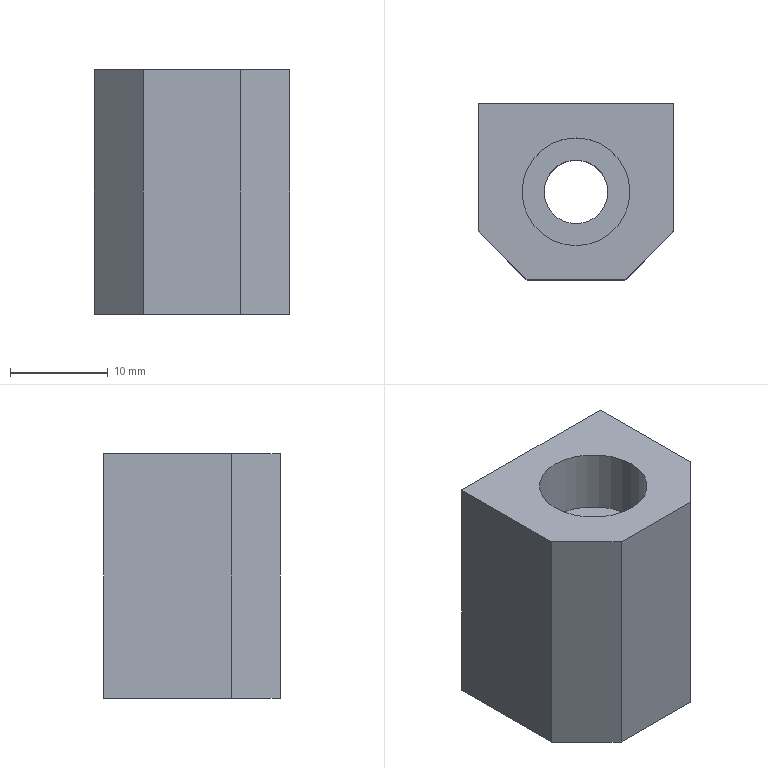Part | STEP file | P011002S004-007 | 1 solid | 11 faces | box 20 x 18 x 25 mm | volume 7143 mm3 | plane 9 | cylinder 2 | commonest cylinder face diameters 6.5 x1 11 x1
STEP:
#1=CARTESIAN_POINT('',(0.,0.,0.));
#2=DIRECTION('',(0.,0.,1.));
#3=DIRECTION('',(1.,0.,0.));
#4=AXIS2_PLACEMENT_3D('',#1,#2,#3);
#5=CARTESIAN_POINT('',(5.,-287.,-23.));
#6=VERTEX_POINT('',#5);
#7=CARTESIAN_POINT('',(-5.,-287.,-23.));
#8=VERTEX_POINT('',#7);
#9=CARTESIAN_POINT('',(-5.,-287.,-23.));
#10=DIRECTION('',(-1.,0.,0.));
#11=VECTOR('',#10,1.);
#12=LINE('',#9,#11);
#13=CARTESIAN_POINT('',(-5.,-274.,-23.));
#14=DIRECTION('',(0.,0.,-1.));
#15=DIRECTION('',(0.,1.,0.));
#16=AXIS2_PLACEMENT_3D('',#13,#14,#15);
#17=PLANE('',#16);
#18=CARTESIAN_POINT('',(-13.,0.));
#19=DIRECTION('',(0.,-1.));
#20=VECTOR('',#19,1.);
#21=LINE('',#18,#20);
#22=(GEOMETRIC_REPRESENTATION_CONTEXT(2)PARAMETRIC_REPRESENTATION_CONTEXT()REPRESENTATION_CONTEXT('',''));
#23=DEFINITIONAL_REPRESENTATION('',(#21),#22);
#24=PCURVE('',#17,#23);
#25=CARTESIAN_POINT('',(-5.,-287.,-23.));
#26=DIRECTION('',(0.,-1.,0.));
#27=DIRECTION('',(0.,0.,-1.));
#28=AXIS2_PLACEMENT_3D('',#25,#26,#27);
#29=PLANE('',#28);
#30=CARTESIAN_POINT('',(0.,0.));
#31=DIRECTION('',(0.,-1.));
#32=VECTOR('',#31,1.);
#33=LINE('',#30,#32);
#34=(GEOMETRIC_REPRESENTATION_CONTEXT(2)PARAMETRIC_REPRESENTATION_CONTEXT()REPRESENTATION_CONTEXT('',''));
#35=DEFINITIONAL_REPRESENTATION('',(#33),#34);
#36=PCURVE('',#29,#35);
#37=SURFACE_CURVE('',#12,(#24,#36),.PCURVE_S1.);
#38=EDGE_CURVE('',#6,#8,#37,.T.);
#39=ORIENTED_EDGE('',*,*,#38,.T.);
#40=CARTESIAN_POINT('',(-10.,-282.,-23.));
#41=VERTEX_POINT('',#40);
#42=CARTESIAN_POINT('',(-11.5,-280.5,-23.));
#43=DIRECTION('',(0.7071,-0.7071,0.));
#44=VECTOR('',#43,1.);
#45=LINE('',#42,#44);
#46=CARTESIAN_POINT('',(-6.5,-6.5));
#47=DIRECTION('',(-0.7071,0.7071));
#48=VECTOR('',#47,1.);
#49=LINE('',#46,#48);
#50=(GEOMETRIC_REPRESENTATION_CONTEXT(2)PARAMETRIC_REPRESENTATION_CONTEXT()REPRESENTATION_CONTEXT('',''));
#51=DEFINITIONAL_REPRESENTATION('',(#49),#50);
#52=PCURVE('',#17,#51);
#53=CARTESIAN_POINT('',(-5.,-287.,-23.));
#54=DIRECTION('',(0.7071,0.7071,0.));
#55=DIRECTION('',(0.7071,-0.7071,0.));
#56=AXIS2_PLACEMENT_3D('',#53,#54,#55);
#57=PLANE('',#56);
#58=CARTESIAN_POINT('',(-9.192,0.));
#59=DIRECTION('',(1.,0.));
#60=VECTOR('',#59,1.);
#61=LINE('',#58,#60);
#62=(GEOMETRIC_REPRESENTATION_CONTEXT(2)PARAMETRIC_REPRESENTATION_CONTEXT()REPRESENTATION_CONTEXT('',''));
#63=DEFINITIONAL_REPRESENTATION('',(#61),#62);
#64=PCURVE('',#57,#63);
#65=SURFACE_CURVE('',#45,(#52,#64),.PCURVE_S1.);
#66=EDGE_CURVE('',#41,#8,#65,.T.);
#67=ORIENTED_EDGE('',*,*,#66,.F.);
#68=CARTESIAN_POINT('',(-10.,-269.,-23.));
#69=VERTEX_POINT('',#68);
#70=CARTESIAN_POINT('',(-10.,-274.,-23.));
#71=DIRECTION('',(0.,1.,0.));
#72=VECTOR('',#71,1.);
#73=LINE('',#70,#72);
#74=CARTESIAN_POINT('',(0.,-5.));
#75=DIRECTION('',(1.,0.));
#76=VECTOR('',#75,1.);
#77=LINE('',#74,#76);
#78=(GEOMETRIC_REPRESENTATION_CONTEXT(2)PARAMETRIC_REPRESENTATION_CONTEXT()REPRESENTATION_CONTEXT('',''));
#79=DEFINITIONAL_REPRESENTATION('',(#77),#78);
#80=PCURVE('',#17,#79);
#81=CARTESIAN_POINT('',(-10.,-274.,-23.));
#82=DIRECTION('',(-1.,0.,0.));
#83=DIRECTION('',(0.,0.,1.));
#84=AXIS2_PLACEMENT_3D('',#81,#82,#83);
#85=PLANE('',#84);
#86=CARTESIAN_POINT('',(0.,0.));
#87=DIRECTION('',(0.,1.));
#88=VECTOR('',#87,1.);
#89=LINE('',#86,#88);
#90=(GEOMETRIC_REPRESENTATION_CONTEXT(2)PARAMETRIC_REPRESENTATION_CONTEXT()REPRESENTATION_CONTEXT('',''));
#91=DEFINITIONAL_REPRESENTATION('',(#89),#90);
#92=PCURVE('',#85,#91);
#93=SURFACE_CURVE('',#73,(#80,#92),.PCURVE_S1.);
#94=EDGE_CURVE('',#41,#69,#93,.T.);
#95=ORIENTED_EDGE('',*,*,#94,.T.);
#96=CARTESIAN_POINT('',(10.,-269.,-23.));
#97=VERTEX_POINT('',#96);
#98=CARTESIAN_POINT('',(-5.,-269.,-23.));
#99=DIRECTION('',(1.,0.,0.));
#100=VECTOR('',#99,1.);
#101=LINE('',#98,#100);
#102=CARTESIAN_POINT('',(5.,0.));
#103=DIRECTION('',(0.,1.));
#104=VECTOR('',#103,1.);
#105=LINE('',#102,#104);
#106=(GEOMETRIC_REPRESENTATION_CONTEXT(2)PARAMETRIC_REPRESENTATION_CONTEXT()REPRESENTATION_CONTEXT('',''));
#107=DEFINITIONAL_REPRESENTATION('',(#105),#106);
#108=PCURVE('',#17,#107);
#109=CARTESIAN_POINT('',(-5.,-269.,-23.));
#110=DIRECTION('',(0.,1.,0.));
#111=DIRECTION('',(0.,0.,1.));
#112=AXIS2_PLACEMENT_3D('',#109,#110,#111);
#113=PLANE('',#112);
#114=CARTESIAN_POINT('',(0.,0.));
#115=DIRECTION('',(0.,1.));
#116=VECTOR('',#115,1.);
#117=LINE('',#114,#116);
#118=(GEOMETRIC_REPRESENTATION_CONTEXT(2)PARAMETRIC_REPRESENTATION_CONTEXT()REPRESENTATION_CONTEXT('',''));
#119=DEFINITIONAL_REPRESENTATION('',(#117),#118);
#120=PCURVE('',#113,#119);
#121=SURFACE_CURVE('',#101,(#108,#120),.PCURVE_S1.);
#122=EDGE_CURVE('',#69,#97,#121,.T.);
#123=ORIENTED_EDGE('',*,*,#122,.T.);
#124=CARTESIAN_POINT('',(10.,-282.,-23.));
#125=VERTEX_POINT('',#124);
#126=CARTESIAN_POINT('',(10.,-274.,-23.));
#127=DIRECTION('',(0.,-1.,0.));
#128=VECTOR('',#127,1.);
#129=LINE('',#126,#128);
#130=CARTESIAN_POINT('',(0.,15.));
#131=DIRECTION('',(-1.,0.));
#132=VECTOR('',#131,1.);
#133=LINE('',#130,#132);
#134=(GEOMETRIC_REPRESENTATION_CONTEXT(2)PARAMETRIC_REPRESENTATION_CONTEXT()REPRESENTATION_CONTEXT('',''));
#135=DEFINITIONAL_REPRESENTATION('',(#133),#134);
#136=PCURVE('',#17,#135);
#137=CARTESIAN_POINT('',(10.,-274.,-23.));
#138=DIRECTION('',(1.,0.,0.));
#139=DIRECTION('',(0.,0.,-1.));
#140=AXIS2_PLACEMENT_3D('',#137,#138,#139);
#141=PLANE('',#140);
#142=CARTESIAN_POINT('',(0.,0.));
#143=DIRECTION('',(0.,-1.));
#144=VECTOR('',#143,1.);
#145=LINE('',#142,#144);
#146=(GEOMETRIC_REPRESENTATION_CONTEXT(2)PARAMETRIC_REPRESENTATION_CONTEXT()REPRESENTATION_CONTEXT('',''));
#147=DEFINITIONAL_REPRESENTATION('',(#145),#146);
#148=PCURVE('',#141,#147);
#149=SURFACE_CURVE('',#129,(#136,#148),.PCURVE_S1.);
#150=EDGE_CURVE('',#97,#125,#149,.T.);
#151=ORIENTED_EDGE('',*,*,#150,.T.);
#152=CARTESIAN_POINT('',(6.5,-285.5,-23.));
#153=DIRECTION('',(0.7071,0.7071,0.));
#154=VECTOR('',#153,1.);
#155=LINE('',#152,#154);
#156=CARTESIAN_POINT('',(-11.5,11.5));
#157=DIRECTION('',(0.7071,0.7071));
#158=VECTOR('',#157,1.);
#159=LINE('',#156,#158);
#160=(GEOMETRIC_REPRESENTATION_CONTEXT(2)PARAMETRIC_REPRESENTATION_CONTEXT()REPRESENTATION_CONTEXT('',''));
#161=DEFINITIONAL_REPRESENTATION('',(#159),#160);
#162=PCURVE('',#17,#161);
#163=CARTESIAN_POINT('',(10.,-282.,-23.));
#164=DIRECTION('',(-0.7071,0.7071,0.));
#165=DIRECTION('',(0.7071,0.7071,0.));
#166=AXIS2_PLACEMENT_3D('',#163,#164,#165);
#167=PLANE('',#166);
#168=CARTESIAN_POINT('',(-4.95,0.));
#169=DIRECTION('',(1.,0.));
#170=VECTOR('',#169,1.);
#171=LINE('',#168,#170);
#172=(GEOMETRIC_REPRESENTATION_CONTEXT(2)PARAMETRIC_REPRESENTATION_CONTEXT()REPRESENTATION_CONTEXT('',''));
#173=DEFINITIONAL_REPRESENTATION('',(#171),#172);
#174=PCURVE('',#167,#173);
#175=SURFACE_CURVE('',#155,(#162,#174),.PCURVE_S1.);
#176=EDGE_CURVE('',#6,#125,#175,.T.);
#177=ORIENTED_EDGE('',*,*,#176,.F.);
#178=EDGE_LOOP('',(#39,#67,#95,#123,#151,#177));
#179=FACE_BOUND('',#178,.T.);
#180=CARTESIAN_POINT('',(3.25,-278.,-23.));
#181=VERTEX_POINT('',#180);
#182=CARTESIAN_POINT('',(0.,-278.,-23.));
#183=DIRECTION('',(0.,0.,-1.));
#184=DIRECTION('',(1.,0.,0.));
#185=AXIS2_PLACEMENT_3D('',#182,#183,#184);
#186=CIRCLE('',#185,3.25);
#187=CARTESIAN_POINT('',(-4.,5.));
#188=DIRECTION('',(0.,1.));
#189=AXIS2_PLACEMENT_2D('',#187,#188);
#190=CIRCLE('',#189,3.25);
#191=(GEOMETRIC_REPRESENTATION_CONTEXT(2)PARAMETRIC_REPRESENTATION_CONTEXT()REPRESENTATION_CONTEXT('',''));
#192=DEFINITIONAL_REPRESENTATION('',(#190),#191);
#193=PCURVE('',#17,#192);
#194=CARTESIAN_POINT('',(0.,-278.,19.));
#195=DIRECTION('',(0.,0.,-1.));
#196=DIRECTION('',(1.,0.,0.));
#197=AXIS2_PLACEMENT_3D('',#194,#195,#196);
#198=CYLINDRICAL_SURFACE('',#197,3.25);
#199=CARTESIAN_POINT('',(0.,42.));
#200=DIRECTION('',(1.,0.));
#201=VECTOR('',#200,1.);
#202=LINE('',#199,#201);
#203=(GEOMETRIC_REPRESENTATION_CONTEXT(2)PARAMETRIC_REPRESENTATION_CONTEXT()REPRESENTATION_CONTEXT('',''));
#204=DEFINITIONAL_REPRESENTATION('',(#202),#203);
#205=PCURVE('',#198,#204);
#206=SURFACE_CURVE('',#186,(#193,#205),.PCURVE_S1.);
#207=EDGE_CURVE('',#181,#181,#206,.T.);
#208=ORIENTED_EDGE('',*,*,#207,.F.);
#209=EDGE_LOOP('',(#208));
#210=FACE_BOUND('',#209,.T.);
#211=ADVANCED_FACE('',(#179,#210),#17,.T.);
#212=CARTESIAN_POINT('',(-5.5,-278.,2.));
#213=VERTEX_POINT('',#212);
#214=CARTESIAN_POINT('',(0.,-278.,2.));
#215=DIRECTION('',(0.,0.,-1.));
#216=DIRECTION('',(-1.,0.,0.));
#217=AXIS2_PLACEMENT_3D('',#214,#215,#216);
#218=CIRCLE('',#217,5.5);
#219=CARTESIAN_POINT('',(-5.,-274.,2.));
#220=DIRECTION('',(0.,0.,1.));
#221=DIRECTION('',(0.,-1.,0.));
#222=AXIS2_PLACEMENT_3D('',#219,#220,#221);
#223=PLANE('',#222);
#224=CARTESIAN_POINT('',(4.,-0.5));
#225=CARTESIAN_POINT('',(-5.526,-0.5));
#226=CARTESIAN_POINT('',(-0.7631,7.75));
#227=CARTESIAN_POINT('',(4.,16.));
#228=CARTESIAN_POINT('',(8.763,7.75));
#229=CARTESIAN_POINT('',(13.526,-0.5));
#230=CARTESIAN_POINT('',(4.,-0.5));
#231=(BOUNDED_CURVE()B_SPLINE_CURVE(2,(#224,#225,#226,#227,#228,#229,#230),.UNSPECIFIED.,.T.,.F.)B_SPLINE_CURVE_WITH_KNOTS((1,2,2,2,2,1),(-2.094,0.,2.094,4.189,6.283,8.378),.UNSPECIFIED.)CURVE()GEOMETRIC_REPRESENTATION_ITEM()RATIONAL_B_SPLINE_CURVE((1.,0.5,1.,0.5,1.,0.5,1.))REPRESENTATION_ITEM(''));
#232=(GEOMETRIC_REPRESENTATION_CONTEXT(2)PARAMETRIC_REPRESENTATION_CONTEXT()REPRESENTATION_CONTEXT('',''));
#233=DEFINITIONAL_REPRESENTATION('',(#231),#232);
#234=PCURVE('',#223,#233);
#235=CARTESIAN_POINT('',(0.,-278.,19.));
#236=DIRECTION('',(0.,0.,-1.));
#237=DIRECTION('',(1.,0.,0.));
#238=AXIS2_PLACEMENT_3D('',#235,#236,#237);
#239=CYLINDRICAL_SURFACE('',#238,5.5);
#240=CARTESIAN_POINT('',(3.142,17.));
#241=DIRECTION('',(1.,0.));
#242=VECTOR('',#241,1.);
#243=LINE('',#240,#242);
#244=(GEOMETRIC_REPRESENTATION_CONTEXT(2)PARAMETRIC_REPRESENTATION_CONTEXT()REPRESENTATION_CONTEXT('',''));
#245=DEFINITIONAL_REPRESENTATION('',(#243),#244);
#246=PCURVE('',#239,#245);
#247=SURFACE_CURVE('',#218,(#234,#246),.PCURVE_S1.);
#248=EDGE_CURVE('',#213,#213,#247,.T.);
#249=ORIENTED_EDGE('',*,*,#248,.T.);
#250=EDGE_LOOP('',(#249));
#251=FACE_BOUND('',#250,.T.);
#252=CARTESIAN_POINT('',(10.,-282.,2.));
#253=VERTEX_POINT('',#252);
#254=CARTESIAN_POINT('',(10.,-269.,2.));
#255=VERTEX_POINT('',#254);
#256=CARTESIAN_POINT('',(10.,-274.,2.));
#257=DIRECTION('',(0.,1.,0.));
#258=VECTOR('',#257,1.);
#259=LINE('',#256,#258);
#260=CARTESIAN_POINT('',(0.,15.));
#261=DIRECTION('',(-1.,0.));
#262=VECTOR('',#261,1.);
#263=LINE('',#260,#262);
#264=(GEOMETRIC_REPRESENTATION_CONTEXT(2)PARAMETRIC_REPRESENTATION_CONTEXT()REPRESENTATION_CONTEXT('',''));
#265=DEFINITIONAL_REPRESENTATION('',(#263),#264);
#266=PCURVE('',#223,#265);
#267=CARTESIAN_POINT('',(-25.,0.));
#268=DIRECTION('',(0.,1.));
#269=VECTOR('',#268,1.);
#270=LINE('',#267,#269);
#271=(GEOMETRIC_REPRESENTATION_CONTEXT(2)PARAMETRIC_REPRESENTATION_CONTEXT()REPRESENTATION_CONTEXT('',''));
#272=DEFINITIONAL_REPRESENTATION('',(#270),#271);
#273=PCURVE('',#141,#272);
#274=SURFACE_CURVE('',#259,(#266,#273),.PCURVE_S1.);
#275=EDGE_CURVE('',#253,#255,#274,.T.);
#276=ORIENTED_EDGE('',*,*,#275,.T.);
#277=CARTESIAN_POINT('',(-10.,-269.,2.));
#278=VERTEX_POINT('',#277);
#279=CARTESIAN_POINT('',(-5.,-269.,2.));
#280=DIRECTION('',(-1.,0.,0.));
#281=VECTOR('',#280,1.);
#282=LINE('',#279,#281);
#283=CARTESIAN_POINT('',(-5.,0.));
#284=DIRECTION('',(0.,-1.));
#285=VECTOR('',#284,1.);
#286=LINE('',#283,#285);
#287=(GEOMETRIC_REPRESENTATION_CONTEXT(2)PARAMETRIC_REPRESENTATION_CONTEXT()REPRESENTATION_CONTEXT('',''));
#288=DEFINITIONAL_REPRESENTATION('',(#286),#287);
#289=PCURVE('',#223,#288);
#290=CARTESIAN_POINT('',(25.,0.));
#291=DIRECTION('',(0.,-1.));
#292=VECTOR('',#291,1.);
#293=LINE('',#290,#292);
#294=(GEOMETRIC_REPRESENTATION_CONTEXT(2)PARAMETRIC_REPRESENTATION_CONTEXT()REPRESENTATION_CONTEXT('',''));
#295=DEFINITIONAL_REPRESENTATION('',(#293),#294);
#296=PCURVE('',#113,#295);
#297=SURFACE_CURVE('',#282,(#289,#296),.PCURVE_S1.);
#298=EDGE_CURVE('',#255,#278,#297,.T.);
#299=ORIENTED_EDGE('',*,*,#298,.T.);
#300=CARTESIAN_POINT('',(-10.,-282.,2.));
#301=VERTEX_POINT('',#300);
#302=CARTESIAN_POINT('',(-10.,-274.,2.));
#303=DIRECTION('',(0.,-1.,0.));
#304=VECTOR('',#303,1.);
#305=LINE('',#302,#304);
#306=CARTESIAN_POINT('',(0.,-5.));
#307=DIRECTION('',(1.,0.));
#308=VECTOR('',#307,1.);
#309=LINE('',#306,#308);
#310=(GEOMETRIC_REPRESENTATION_CONTEXT(2)PARAMETRIC_REPRESENTATION_CONTEXT()REPRESENTATION_CONTEXT('',''));
#311=DEFINITIONAL_REPRESENTATION('',(#309),#310);
#312=PCURVE('',#223,#311);
#313=CARTESIAN_POINT('',(25.,0.));
#314=DIRECTION('',(0.,-1.));
#315=VECTOR('',#314,1.);
#316=LINE('',#313,#315);
#317=(GEOMETRIC_REPRESENTATION_CONTEXT(2)PARAMETRIC_REPRESENTATION_CONTEXT()REPRESENTATION_CONTEXT('',''));
#318=DEFINITIONAL_REPRESENTATION('',(#316),#317);
#319=PCURVE('',#85,#318);
#320=SURFACE_CURVE('',#305,(#312,#319),.PCURVE_S1.);
#321=EDGE_CURVE('',#278,#301,#320,.T.);
#322=ORIENTED_EDGE('',*,*,#321,.T.);
#323=CARTESIAN_POINT('',(-5.,-287.,2.));
#324=VERTEX_POINT('',#323);
#325=CARTESIAN_POINT('',(-11.5,-280.5,2.));
#326=DIRECTION('',(-0.7071,0.7071,0.));
#327=VECTOR('',#326,1.);
#328=LINE('',#325,#327);
#329=CARTESIAN_POINT('',(6.5,-6.5));
#330=DIRECTION('',(-0.7071,-0.7071));
#331=VECTOR('',#330,1.);
#332=LINE('',#329,#331);
#333=(GEOMETRIC_REPRESENTATION_CONTEXT(2)PARAMETRIC_REPRESENTATION_CONTEXT()REPRESENTATION_CONTEXT('',''));
#334=DEFINITIONAL_REPRESENTATION('',(#332),#333);
#335=PCURVE('',#223,#334);
#336=CARTESIAN_POINT('',(-9.192,-25.));
#337=DIRECTION('',(-1.,0.));
#338=VECTOR('',#337,1.);
#339=LINE('',#336,#338);
#340=(GEOMETRIC_REPRESENTATION_CONTEXT(2)PARAMETRIC_REPRESENTATION_CONTEXT()REPRESENTATION_CONTEXT('',''));
#341=DEFINITIONAL_REPRESENTATION('',(#339),#340);
#342=PCURVE('',#57,#341);
#343=SURFACE_CURVE('',#328,(#335,#342),.PCURVE_S1.);
#344=EDGE_CURVE('',#324,#301,#343,.T.);
#345=ORIENTED_EDGE('',*,*,#344,.F.);
#346=CARTESIAN_POINT('',(5.,-287.,2.));
#347=VERTEX_POINT('',#346);
#348=CARTESIAN_POINT('',(-5.,-287.,2.));
#349=DIRECTION('',(1.,0.,0.));
#350=VECTOR('',#349,1.);
#351=LINE('',#348,#350);
#352=CARTESIAN_POINT('',(13.,0.));
#353=DIRECTION('',(0.,1.));
#354=VECTOR('',#353,1.);
#355=LINE('',#352,#354);
#356=(GEOMETRIC_REPRESENTATION_CONTEXT(2)PARAMETRIC_REPRESENTATION_CONTEXT()REPRESENTATION_CONTEXT('',''));
#357=DEFINITIONAL_REPRESENTATION('',(#355),#356);
#358=PCURVE('',#223,#357);
#359=CARTESIAN_POINT('',(-25.,0.));
#360=DIRECTION('',(0.,1.));
#361=VECTOR('',#360,1.);
#362=LINE('',#359,#361);
#363=(GEOMETRIC_REPRESENTATION_CONTEXT(2)PARAMETRIC_REPRESENTATION_CONTEXT()REPRESENTATION_CONTEXT('',''));
#364=DEFINITIONAL_REPRESENTATION('',(#362),#363);
#365=PCURVE('',#29,#364);
#366=SURFACE_CURVE('',#351,(#358,#365),.PCURVE_S1.);
#367=EDGE_CURVE('',#324,#347,#366,.T.);
#368=ORIENTED_EDGE('',*,*,#367,.T.);
#369=CARTESIAN_POINT('',(6.5,-285.5,2.));
#370=DIRECTION('',(-0.7071,-0.7071,0.));
#371=VECTOR('',#370,1.);
#372=LINE('',#369,#371);
#373=CARTESIAN_POINT('',(11.5,11.5));
#374=DIRECTION('',(0.7071,-0.7071));
#375=VECTOR('',#374,1.);
#376=LINE('',#373,#375);
#377=(GEOMETRIC_REPRESENTATION_CONTEXT(2)PARAMETRIC_REPRESENTATION_CONTEXT()REPRESENTATION_CONTEXT('',''));
#378=DEFINITIONAL_REPRESENTATION('',(#376),#377);
#379=PCURVE('',#223,#378);
#380=CARTESIAN_POINT('',(-4.95,-25.));
#381=DIRECTION('',(-1.,0.));
#382=VECTOR('',#381,1.);
#383=LINE('',#380,#382);
#384=(GEOMETRIC_REPRESENTATION_CONTEXT(2)PARAMETRIC_REPRESENTATION_CONTEXT()REPRESENTATION_CONTEXT('',''));
#385=DEFINITIONAL_REPRESENTATION('',(#383),#384);
#386=PCURVE('',#167,#385);
#387=SURFACE_CURVE('',#372,(#379,#386),.PCURVE_S1.);
#388=EDGE_CURVE('',#253,#347,#387,.T.);
#389=ORIENTED_EDGE('',*,*,#388,.F.);
#390=EDGE_LOOP('',(#276,#299,#322,#345,#368,#389));
#391=FACE_BOUND('',#390,.T.);
#392=ADVANCED_FACE('',(#251,#391),#223,.T.);
#393=ORIENTED_EDGE('',*,*,#150,.F.);
#394=CARTESIAN_POINT('',(10.,-269.,-23.));
#395=DIRECTION('',(0.,0.,1.));
#396=VECTOR('',#395,1.);
#397=LINE('',#394,#396);
#398=CARTESIAN_POINT('',(0.,5.));
#399=DIRECTION('',(-1.,0.));
#400=VECTOR('',#399,1.);
#401=LINE('',#398,#400);
#402=(GEOMETRIC_REPRESENTATION_CONTEXT(2)PARAMETRIC_REPRESENTATION_CONTEXT()REPRESENTATION_CONTEXT('',''));
#403=DEFINITIONAL_REPRESENTATION('',(#401),#402);
#404=PCURVE('',#141,#403);
#405=CARTESIAN_POINT('',(0.,15.));
#406=DIRECTION('',(1.,0.));
#407=VECTOR('',#406,1.);
#408=LINE('',#405,#407);
#409=(GEOMETRIC_REPRESENTATION_CONTEXT(2)PARAMETRIC_REPRESENTATION_CONTEXT()REPRESENTATION_CONTEXT('',''));
#410=DEFINITIONAL_REPRESENTATION('',(#408),#409);
#411=PCURVE('',#113,#410);
#412=SURFACE_CURVE('',#397,(#404,#411),.PCURVE_S1.);
#413=EDGE_CURVE('',#97,#255,#412,.T.);
#414=ORIENTED_EDGE('',*,*,#413,.T.);
#415=ORIENTED_EDGE('',*,*,#275,.F.);
#416=CARTESIAN_POINT('',(10.,-282.,-23.));
#417=DIRECTION('',(0.,0.,1.));
#418=VECTOR('',#417,1.);
#419=LINE('',#416,#418);
#420=CARTESIAN_POINT('',(0.,-8.));
#421=DIRECTION('',(-1.,0.));
#422=VECTOR('',#421,1.);
#423=LINE('',#420,#422);
#424=(GEOMETRIC_REPRESENTATION_CONTEXT(2)PARAMETRIC_REPRESENTATION_CONTEXT()REPRESENTATION_CONTEXT('',''));
#425=DEFINITIONAL_REPRESENTATION('',(#423),#424);
#426=PCURVE('',#141,#425);
#427=CARTESIAN_POINT('',(0.,0.));
#428=DIRECTION('',(0.,-1.));
#429=VECTOR('',#428,1.);
#430=LINE('',#427,#429);
#431=(GEOMETRIC_REPRESENTATION_CONTEXT(2)PARAMETRIC_REPRESENTATION_CONTEXT()REPRESENTATION_CONTEXT('',''));
#432=DEFINITIONAL_REPRESENTATION('',(#430),#431);
#433=PCURVE('',#167,#432);
#434=SURFACE_CURVE('',#419,(#426,#433),.PCURVE_S1.);
#435=EDGE_CURVE('',#125,#253,#434,.T.);
#436=ORIENTED_EDGE('',*,*,#435,.F.);
#437=EDGE_LOOP('',(#393,#414,#415,#436));
#438=FACE_BOUND('',#437,.T.);
#439=ADVANCED_FACE('',(#438),#141,.T.);
#440=ORIENTED_EDGE('',*,*,#413,.F.);
#441=ORIENTED_EDGE('',*,*,#122,.F.);
#442=CARTESIAN_POINT('',(-10.,-269.,-23.));
#443=DIRECTION('',(0.,0.,1.));
#444=VECTOR('',#443,1.);
#445=LINE('',#442,#444);
#446=CARTESIAN_POINT('',(0.,-5.));
#447=DIRECTION('',(1.,0.));
#448=VECTOR('',#447,1.);
#449=LINE('',#446,#448);
#450=(GEOMETRIC_REPRESENTATION_CONTEXT(2)PARAMETRIC_REPRESENTATION_CONTEXT()REPRESENTATION_CONTEXT('',''));
#451=DEFINITIONAL_REPRESENTATION('',(#449),#450);
#452=PCURVE('',#113,#451);
#453=CARTESIAN_POINT('',(0.,5.));
#454=DIRECTION('',(1.,0.));
#455=VECTOR('',#454,1.);
#456=LINE('',#453,#455);
#457=(GEOMETRIC_REPRESENTATION_CONTEXT(2)PARAMETRIC_REPRESENTATION_CONTEXT()REPRESENTATION_CONTEXT('',''));
#458=DEFINITIONAL_REPRESENTATION('',(#456),#457);
#459=PCURVE('',#85,#458);
#460=SURFACE_CURVE('',#445,(#452,#459),.PCURVE_S1.);
#461=EDGE_CURVE('',#69,#278,#460,.T.);
#462=ORIENTED_EDGE('',*,*,#461,.T.);
#463=ORIENTED_EDGE('',*,*,#298,.F.);
#464=EDGE_LOOP('',(#440,#441,#462,#463));
#465=FACE_BOUND('',#464,.T.);
#466=ADVANCED_FACE('',(#465),#113,.T.);
#467=ORIENTED_EDGE('',*,*,#321,.F.);
#468=ORIENTED_EDGE('',*,*,#461,.F.);
#469=ORIENTED_EDGE('',*,*,#94,.F.);
#470=CARTESIAN_POINT('',(-10.,-282.,-23.));
#471=DIRECTION('',(0.,0.,-1.));
#472=VECTOR('',#471,1.);
#473=LINE('',#470,#472);
#474=CARTESIAN_POINT('',(0.,-8.));
#475=DIRECTION('',(-1.,0.));
#476=VECTOR('',#475,1.);
#477=LINE('',#474,#476);
#478=(GEOMETRIC_REPRESENTATION_CONTEXT(2)PARAMETRIC_REPRESENTATION_CONTEXT()REPRESENTATION_CONTEXT('',''));
#479=DEFINITIONAL_REPRESENTATION('',(#477),#478);
#480=PCURVE('',#85,#479);
#481=CARTESIAN_POINT('',(-7.071,0.));
#482=DIRECTION('',(0.,1.));
#483=VECTOR('',#482,1.);
#484=LINE('',#481,#483);
#485=(GEOMETRIC_REPRESENTATION_CONTEXT(2)PARAMETRIC_REPRESENTATION_CONTEXT()REPRESENTATION_CONTEXT('',''));
#486=DEFINITIONAL_REPRESENTATION('',(#484),#485);
#487=PCURVE('',#57,#486);
#488=SURFACE_CURVE('',#473,(#480,#487),.PCURVE_S1.);
#489=EDGE_CURVE('',#301,#41,#488,.T.);
#490=ORIENTED_EDGE('',*,*,#489,.F.);
#491=EDGE_LOOP('',(#467,#468,#469,#490));
#492=FACE_BOUND('',#491,.T.);
#493=ADVANCED_FACE('',(#492),#85,.T.);
#494=ORIENTED_EDGE('',*,*,#367,.F.);
#495=CARTESIAN_POINT('',(-5.,-287.,-23.));
#496=DIRECTION('',(0.,0.,1.));
#497=VECTOR('',#496,1.);
#498=LINE('',#495,#497);
#499=CARTESIAN_POINT('',(0.,0.));
#500=DIRECTION('',(-1.,0.));
#501=VECTOR('',#500,1.);
#502=LINE('',#499,#501);
#503=(GEOMETRIC_REPRESENTATION_CONTEXT(2)PARAMETRIC_REPRESENTATION_CONTEXT()REPRESENTATION_CONTEXT('',''));
#504=DEFINITIONAL_REPRESENTATION('',(#502),#503);
#505=PCURVE('',#29,#504);
#506=CARTESIAN_POINT('',(0.,0.));
#507=DIRECTION('',(0.,-1.));
#508=VECTOR('',#507,1.);
#509=LINE('',#506,#508);
#510=(GEOMETRIC_REPRESENTATION_CONTEXT(2)PARAMETRIC_REPRESENTATION_CONTEXT()REPRESENTATION_CONTEXT('',''));
#511=DEFINITIONAL_REPRESENTATION('',(#509),#510);
#512=PCURVE('',#57,#511);
#513=SURFACE_CURVE('',#498,(#505,#512),.PCURVE_S1.);
#514=EDGE_CURVE('',#8,#324,#513,.T.);
#515=ORIENTED_EDGE('',*,*,#514,.F.);
#516=ORIENTED_EDGE('',*,*,#38,.F.);
#517=CARTESIAN_POINT('',(5.,-287.,-23.));
#518=DIRECTION('',(0.,0.,-1.));
#519=VECTOR('',#518,1.);
#520=LINE('',#517,#519);
#521=CARTESIAN_POINT('',(0.,10.));
#522=DIRECTION('',(1.,0.));
#523=VECTOR('',#522,1.);
#524=LINE('',#521,#523);
#525=(GEOMETRIC_REPRESENTATION_CONTEXT(2)PARAMETRIC_REPRESENTATION_CONTEXT()REPRESENTATION_CONTEXT('',''));
#526=DEFINITIONAL_REPRESENTATION('',(#524),#525);
#527=PCURVE('',#29,#526);
#528=CARTESIAN_POINT('',(-7.071,0.));
#529=DIRECTION('',(0.,1.));
#530=VECTOR('',#529,1.);
#531=LINE('',#528,#530);
#532=(GEOMETRIC_REPRESENTATION_CONTEXT(2)PARAMETRIC_REPRESENTATION_CONTEXT()REPRESENTATION_CONTEXT('',''));
#533=DEFINITIONAL_REPRESENTATION('',(#531),#532);
#534=PCURVE('',#167,#533);
#535=SURFACE_CURVE('',#520,(#527,#534),.PCURVE_S1.);
#536=EDGE_CURVE('',#347,#6,#535,.T.);
#537=ORIENTED_EDGE('',*,*,#536,.F.);
#538=EDGE_LOOP('',(#494,#515,#516,#537));
#539=FACE_BOUND('',#538,.T.);
#540=ADVANCED_FACE('',(#539),#29,.T.);
#541=ORIENTED_EDGE('',*,*,#176,.T.);
#542=ORIENTED_EDGE('',*,*,#435,.T.);
#543=ORIENTED_EDGE('',*,*,#388,.T.);
#544=ORIENTED_EDGE('',*,*,#536,.T.);
#545=EDGE_LOOP('',(#541,#542,#543,#544));
#546=FACE_BOUND('',#545,.T.);
#547=ADVANCED_FACE('',(#546),#167,.F.);
#548=ORIENTED_EDGE('',*,*,#66,.T.);
#549=ORIENTED_EDGE('',*,*,#514,.T.);
#550=ORIENTED_EDGE('',*,*,#344,.T.);
#551=ORIENTED_EDGE('',*,*,#489,.T.);
#552=EDGE_LOOP('',(#548,#549,#550,#551));
#553=FACE_BOUND('',#552,.T.);
#554=ADVANCED_FACE('',(#553),#57,.F.);
#555=ORIENTED_EDGE('',*,*,#207,.F.);
#556=CARTESIAN_POINT('',(3.25,-278.,-4.5));
#557=VERTEX_POINT('',#556);
#558=CARTESIAN_POINT('',(3.25,-278.,-4.5));
#559=CARTESIAN_POINT('',(3.25,-278.,-23.));
#560=B_SPLINE_CURVE_WITH_KNOTS('',1,(#558,#559),.UNSPECIFIED.,.F.,.F.,(2,2),(23.5,42.),.PIECEWISE_BEZIER_KNOTS.);
#561=CARTESIAN_POINT('',(0.,0.));
#562=DIRECTION('',(0.,1.));
#563=VECTOR('',#562,1.);
#564=LINE('',#561,#563);
#565=(GEOMETRIC_REPRESENTATION_CONTEXT(2)PARAMETRIC_REPRESENTATION_CONTEXT()REPRESENTATION_CONTEXT('',''));
#566=DEFINITIONAL_REPRESENTATION('',(#564),#565);
#567=PCURVE('',#198,#566);
#568=CARTESIAN_POINT('',(6.283,0.));
#569=DIRECTION('',(0.,1.));
#570=VECTOR('',#569,1.);
#571=LINE('',#568,#570);
#572=(GEOMETRIC_REPRESENTATION_CONTEXT(2)PARAMETRIC_REPRESENTATION_CONTEXT()REPRESENTATION_CONTEXT('',''));
#573=DEFINITIONAL_REPRESENTATION('',(#571),#572);
#574=PCURVE('',#198,#573);
#575=SEAM_CURVE('',#560,(#567,#574),.PCURVE_S1.);
#576=EDGE_CURVE('',#557,#181,#575,.T.);
#577=ORIENTED_EDGE('',*,*,#576,.F.);
#578=CARTESIAN_POINT('',(-3.25,-278.,-4.5));
#579=VERTEX_POINT('',#578);
#580=CARTESIAN_POINT('',(0.,-278.,-4.5));
#581=DIRECTION('',(0.,0.,-1.));
#582=DIRECTION('',(-1.,0.,0.));
#583=AXIS2_PLACEMENT_3D('',#580,#581,#582);
#584=CIRCLE('',#583,3.25);
#585=CARTESIAN_POINT('',(-3.142,23.5));
#586=DIRECTION('',(1.,0.));
#587=VECTOR('',#586,1.);
#588=LINE('',#585,#587);
#589=(GEOMETRIC_REPRESENTATION_CONTEXT(2)PARAMETRIC_REPRESENTATION_CONTEXT()REPRESENTATION_CONTEXT('',''));
#590=DEFINITIONAL_REPRESENTATION('',(#588),#589);
#591=PCURVE('',#198,#590);
#592=CARTESIAN_POINT('',(0.,-278.,-4.5));
#593=DIRECTION('',(0.,0.,1.));
#594=DIRECTION('',(-1.,0.,0.));
#595=AXIS2_PLACEMENT_3D('',#592,#593,#594);
#596=PLANE('',#595);
#597=CARTESIAN_POINT('',(3.25,0.));
#598=CARTESIAN_POINT('',(3.25,-5.629));
#599=CARTESIAN_POINT('',(-1.625,-2.815));
#600=CARTESIAN_POINT('',(-6.5,0.));
#601=CARTESIAN_POINT('',(-1.625,2.815));
#602=CARTESIAN_POINT('',(3.25,5.629));
#603=CARTESIAN_POINT('',(3.25,0.));
#604=(BOUNDED_CURVE()B_SPLINE_CURVE(2,(#597,#598,#599,#600,#601,#602,#603),.UNSPECIFIED.,.T.,.F.)B_SPLINE_CURVE_WITH_KNOTS((1,2,2,2,2,1),(-2.094,0.,2.094,4.189,6.283,8.378),.UNSPECIFIED.)CURVE()GEOMETRIC_REPRESENTATION_ITEM()RATIONAL_B_SPLINE_CURVE((1.,0.5,1.,0.5,1.,0.5,1.))REPRESENTATION_ITEM(''));
#605=(GEOMETRIC_REPRESENTATION_CONTEXT(2)PARAMETRIC_REPRESENTATION_CONTEXT()REPRESENTATION_CONTEXT('',''));
#606=DEFINITIONAL_REPRESENTATION('',(#604),#605);
#607=PCURVE('',#596,#606);
#608=SURFACE_CURVE('',#584,(#591,#607),.PCURVE_S1.);
#609=EDGE_CURVE('',#557,#579,#608,.T.);
#610=ORIENTED_EDGE('',*,*,#609,.T.);
#611=CARTESIAN_POINT('',(0.,-278.,-4.5));
#612=DIRECTION('',(0.,0.,-1.));
#613=DIRECTION('',(-1.,0.,0.));
#614=AXIS2_PLACEMENT_3D('',#611,#612,#613);
#615=CIRCLE('',#614,3.25);
#616=CARTESIAN_POINT('',(3.142,23.5));
#617=DIRECTION('',(1.,0.));
#618=VECTOR('',#617,1.);
#619=LINE('',#616,#618);
#620=(GEOMETRIC_REPRESENTATION_CONTEXT(2)PARAMETRIC_REPRESENTATION_CONTEXT()REPRESENTATION_CONTEXT('',''));
#621=DEFINITIONAL_REPRESENTATION('',(#619),#620);
#622=PCURVE('',#198,#621);
#623=CARTESIAN_POINT('',(3.25,0.));
#624=CARTESIAN_POINT('',(3.25,-5.629));
#625=CARTESIAN_POINT('',(-1.625,-2.815));
#626=CARTESIAN_POINT('',(-6.5,0.));
#627=CARTESIAN_POINT('',(-1.625,2.815));
#628=CARTESIAN_POINT('',(3.25,5.629));
#629=CARTESIAN_POINT('',(3.25,0.));
#630=(BOUNDED_CURVE()B_SPLINE_CURVE(2,(#623,#624,#625,#626,#627,#628,#629),.UNSPECIFIED.,.T.,.F.)B_SPLINE_CURVE_WITH_KNOTS((1,2,2,2,2,1),(-2.094,0.,2.094,4.189,6.283,8.378),.UNSPECIFIED.)CURVE()GEOMETRIC_REPRESENTATION_ITEM()RATIONAL_B_SPLINE_CURVE((1.,0.5,1.,0.5,1.,0.5,1.))REPRESENTATION_ITEM(''));
#631=(GEOMETRIC_REPRESENTATION_CONTEXT(2)PARAMETRIC_REPRESENTATION_CONTEXT()REPRESENTATION_CONTEXT('',''));
#632=DEFINITIONAL_REPRESENTATION('',(#630),#631);
#633=PCURVE('',#596,#632);
#634=SURFACE_CURVE('',#615,(#622,#633),.PCURVE_S1.);
#635=EDGE_CURVE('',#579,#557,#634,.T.);
#636=ORIENTED_EDGE('',*,*,#635,.T.);
#637=ORIENTED_EDGE('',*,*,#576,.T.);
#638=EDGE_LOOP('',(#555,#577,#610,#636,#637));
#639=FACE_BOUND('',#638,.F.);
#640=ADVANCED_FACE('',(#639),#198,.F.);
#641=CARTESIAN_POINT('',(-5.5,-278.,-4.5));
#642=VERTEX_POINT('',#641);
#643=CARTESIAN_POINT('',(0.,-278.,-4.5));
#644=DIRECTION('',(0.,0.,-1.));
#645=DIRECTION('',(-1.,0.,0.));
#646=AXIS2_PLACEMENT_3D('',#643,#644,#645);
#647=CIRCLE('',#646,5.5);
#648=CARTESIAN_POINT('',(5.5,0.));
#649=CARTESIAN_POINT('',(5.5,-9.526));
#650=CARTESIAN_POINT('',(-2.75,-4.763));
#651=CARTESIAN_POINT('',(-11.,0.));
#652=CARTESIAN_POINT('',(-2.75,4.763));
#653=CARTESIAN_POINT('',(5.5,9.526));
#654=CARTESIAN_POINT('',(5.5,0.));
#655=(BOUNDED_CURVE()B_SPLINE_CURVE(2,(#648,#649,#650,#651,#652,#653,#654),.UNSPECIFIED.,.T.,.F.)B_SPLINE_CURVE_WITH_KNOTS((1,2,2,2,2,1),(-2.094,0.,2.094,4.189,6.283,8.378),.UNSPECIFIED.)CURVE()GEOMETRIC_REPRESENTATION_ITEM()RATIONAL_B_SPLINE_CURVE((1.,0.5,1.,0.5,1.,0.5,1.))REPRESENTATION_ITEM(''));
#656=(GEOMETRIC_REPRESENTATION_CONTEXT(2)PARAMETRIC_REPRESENTATION_CONTEXT()REPRESENTATION_CONTEXT('',''));
#657=DEFINITIONAL_REPRESENTATION('',(#655),#656);
#658=PCURVE('',#596,#657);
#659=CARTESIAN_POINT('',(3.142,23.5));
#660=DIRECTION('',(1.,0.));
#661=VECTOR('',#660,1.);
#662=LINE('',#659,#661);
#663=(GEOMETRIC_REPRESENTATION_CONTEXT(2)PARAMETRIC_REPRESENTATION_CONTEXT()REPRESENTATION_CONTEXT('',''));
#664=DEFINITIONAL_REPRESENTATION('',(#662),#663);
#665=PCURVE('',#239,#664);
#666=SURFACE_CURVE('',#647,(#658,#665),.PCURVE_S1.);
#667=EDGE_CURVE('',#642,#642,#666,.T.);
#668=ORIENTED_EDGE('',*,*,#667,.F.);
#669=EDGE_LOOP('',(#668));
#670=FACE_BOUND('',#669,.T.);
#671=ORIENTED_EDGE('',*,*,#635,.T.);
#672=ORIENTED_EDGE('',*,*,#609,.T.);
#673=EDGE_LOOP('',(#671,#672));
#674=FACE_BOUND('',#673,.T.);
#675=ADVANCED_FACE('',(#670,#674),#596,.T.);
#676=ORIENTED_EDGE('',*,*,#667,.F.);
#677=CARTESIAN_POINT('',(-5.5,-278.,2.));
#678=CARTESIAN_POINT('',(-5.5,-278.,-4.5));
#679=B_SPLINE_CURVE_WITH_KNOTS('',1,(#677,#678),.UNSPECIFIED.,.F.,.F.,(2,2),(17.,23.5),.PIECEWISE_BEZIER_KNOTS.);
#680=CARTESIAN_POINT('',(3.142,0.));
#681=DIRECTION('',(0.,1.));
#682=VECTOR('',#681,1.);
#683=LINE('',#680,#682);
#684=(GEOMETRIC_REPRESENTATION_CONTEXT(2)PARAMETRIC_REPRESENTATION_CONTEXT()REPRESENTATION_CONTEXT('',''));
#685=DEFINITIONAL_REPRESENTATION('',(#683),#684);
#686=PCURVE('',#239,#685);
#687=CARTESIAN_POINT('',(9.425,0.));
#688=DIRECTION('',(0.,1.));
#689=VECTOR('',#688,1.);
#690=LINE('',#687,#689);
#691=(GEOMETRIC_REPRESENTATION_CONTEXT(2)PARAMETRIC_REPRESENTATION_CONTEXT()REPRESENTATION_CONTEXT('',''));
#692=DEFINITIONAL_REPRESENTATION('',(#690),#691);
#693=PCURVE('',#239,#692);
#694=SEAM_CURVE('',#679,(#686,#693),.PCURVE_S1.);
#695=EDGE_CURVE('',#213,#642,#694,.T.);
#696=ORIENTED_EDGE('',*,*,#695,.F.);
#697=ORIENTED_EDGE('',*,*,#248,.T.);
#698=ORIENTED_EDGE('',*,*,#695,.T.);
#699=EDGE_LOOP('',(#676,#696,#697,#698));
#700=FACE_BOUND('',#699,.F.);
#701=ADVANCED_FACE('',(#700),#239,.F.);
#702=CLOSED_SHELL('',(#211,#392,#439,#466,#493,#540,#547,#554,#640,#675,#701));
#703=MANIFOLD_SOLID_BREP('',#702);
#704=(LENGTH_UNIT()NAMED_UNIT(*)SI_UNIT(.MILLI.,.METRE.));
#705=UNCERTAINTY_MEASURE_WITH_UNIT(LENGTH_MEASURE(0.000002),#704,'','');
#706=(NAMED_UNIT(*)PLANE_ANGLE_UNIT()SI_UNIT($,.RADIAN.));
#707=(NAMED_UNIT(*)SI_UNIT($,.STERADIAN.)SOLID_ANGLE_UNIT());
#708=(GEOMETRIC_REPRESENTATION_CONTEXT(3)GLOBAL_UNCERTAINTY_ASSIGNED_CONTEXT((#705))GLOBAL_UNIT_ASSIGNED_CONTEXT((#704,#706,#707))REPRESENTATION_CONTEXT('',''));
#709=ADVANCED_BREP_SHAPE_REPRESENTATION('',(#4,#703),#708);